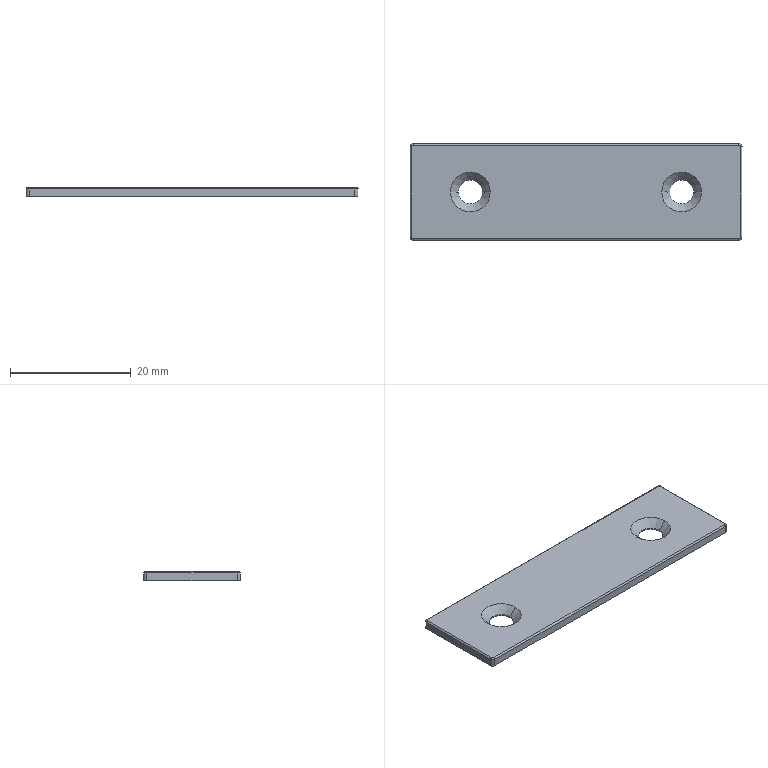Part | SolidWorks | features BaseBody 1 | 1 solid | 26 faces | box 55 x 16 x 1.5 mm | volume 1254 mm3 | cylinder 12 | plane 6 | cone 4 | torus 2 | spline 2 | commonest cylinder face diameters 0.5 x4 1 x4 4 x4
STEP:
#1=CARTESIAN_POINT('',(-15.5,0.,0.2));
#2=VERTEX_POINT('',#1);
#3=CARTESIAN_POINT('',(-19.5,0.,0.2));
#4=VERTEX_POINT('',#3);
#5=CARTESIAN_POINT('',(-17.5,0.,0.2));
#6=DIRECTION('',(0.,0.,-1.));
#7=DIRECTION('',(-1.,0.,0.));
#8=AXIS2_PLACEMENT_3D('',#5,#6,#7);
#9=CIRCLE('',#8,2.);
#10=EDGE_CURVE('',#2,#4,#9,.T.);
#11=ORIENTED_EDGE('',*,*,#10,.F.);
#12=CARTESIAN_POINT('',(-15.5,0.,0.));
#13=VERTEX_POINT('',#12);
#14=CARTESIAN_POINT('',(-15.5,0.,1.5));
#15=DIRECTION('',(0.,0.,-1.));
#16=VECTOR('',#15,1000.);
#17=LINE('',#14,#16);
#18=EDGE_CURVE('',#2,#13,#17,.T.);
#19=ORIENTED_EDGE('',*,*,#18,.T.);
#20=CARTESIAN_POINT('',(-19.5,0.,0.));
#21=VERTEX_POINT('',#20);
#22=CARTESIAN_POINT('',(-17.5,0.,0.));
#23=DIRECTION('',(0.,0.,-1.));
#24=DIRECTION('',(-1.,0.,0.));
#25=AXIS2_PLACEMENT_3D('',#22,#23,#24);
#26=CIRCLE('',#25,2.);
#27=EDGE_CURVE('',#13,#21,#26,.T.);
#28=ORIENTED_EDGE('',*,*,#27,.T.);
#29=CARTESIAN_POINT('',(-19.5,0.,1.5));
#30=DIRECTION('',(0.,0.,-1.));
#31=VECTOR('',#30,1000.);
#32=LINE('',#29,#31);
#33=EDGE_CURVE('',#4,#21,#32,.T.);
#34=ORIENTED_EDGE('',*,*,#33,.F.);
#35=EDGE_LOOP('',(#11,#19,#28,#34));
#36=FACE_OUTER_BOUND('',#35,.T.);
#37=CARTESIAN_POINT('',(-17.5,0.,1.5));
#38=DIRECTION('',(0.,0.,-1.));
#39=DIRECTION('',(-1.,0.,0.));
#40=AXIS2_PLACEMENT_3D('',#37,#38,#39);
#41=CYLINDRICAL_SURFACE('',#40,2.);
#42=ADVANCED_FACE('',(#36),#41,.F.);
#43=CARTESIAN_POINT('',(19.5,0.,0.2));
#44=VERTEX_POINT('',#43);
#45=CARTESIAN_POINT('',(15.5,0.,0.2));
#46=VERTEX_POINT('',#45);
#47=CARTESIAN_POINT('',(17.5,0.,0.2));
#48=DIRECTION('',(0.,0.,-1.));
#49=DIRECTION('',(-1.,0.,0.));
#50=AXIS2_PLACEMENT_3D('',#47,#48,#49);
#51=CIRCLE('',#50,2.);
#52=EDGE_CURVE('',#44,#46,#51,.T.);
#53=ORIENTED_EDGE('',*,*,#52,.F.);
#54=CARTESIAN_POINT('',(19.5,0.,0.));
#55=VERTEX_POINT('',#54);
#56=CARTESIAN_POINT('',(19.5,0.,1.5));
#57=DIRECTION('',(0.,0.,-1.));
#58=VECTOR('',#57,1000.);
#59=LINE('',#56,#58);
#60=EDGE_CURVE('',#44,#55,#59,.T.);
#61=ORIENTED_EDGE('',*,*,#60,.T.);
#62=CARTESIAN_POINT('',(15.5,0.,0.));
#63=VERTEX_POINT('',#62);
#64=CARTESIAN_POINT('',(17.5,0.,0.));
#65=DIRECTION('',(0.,0.,-1.));
#66=DIRECTION('',(-1.,0.,0.));
#67=AXIS2_PLACEMENT_3D('',#64,#65,#66);
#68=CIRCLE('',#67,2.);
#69=EDGE_CURVE('',#55,#63,#68,.T.);
#70=ORIENTED_EDGE('',*,*,#69,.T.);
#71=CARTESIAN_POINT('',(15.5,0.,1.5));
#72=DIRECTION('',(0.,0.,-1.));
#73=VECTOR('',#72,1000.);
#74=LINE('',#71,#73);
#75=EDGE_CURVE('',#46,#63,#74,.T.);
#76=ORIENTED_EDGE('',*,*,#75,.F.);
#77=EDGE_LOOP('',(#53,#61,#70,#76));
#78=FACE_OUTER_BOUND('',#77,.T.);
#79=CARTESIAN_POINT('',(17.5,0.,1.5));
#80=DIRECTION('',(0.,0.,-1.));
#81=DIRECTION('',(-1.,0.,0.));
#82=AXIS2_PLACEMENT_3D('',#79,#80,#81);
#83=CYLINDRICAL_SURFACE('',#82,2.);
#84=ADVANCED_FACE('',(#78),#83,.F.);
#85=ORIENTED_EDGE('',*,*,#10,.T.);
#86=CARTESIAN_POINT('',(-20.8,0.,1.5));
#87=VERTEX_POINT('',#86);
#88=CARTESIAN_POINT('',(-20.8,0.,1.5));
#89=DIRECTION('',(-0.7071,0.,0.7071));
#90=VECTOR('',#89,1000.);
#91=LINE('',#88,#90);
#92=EDGE_CURVE('',#4,#87,#91,.T.);
#93=ORIENTED_EDGE('',*,*,#92,.T.);
#94=CARTESIAN_POINT('',(-14.2,0.,1.5));
#95=VERTEX_POINT('',#94);
#96=CARTESIAN_POINT('',(-17.5,0.,1.5));
#97=DIRECTION('',(0.,0.,-1.));
#98=DIRECTION('',(1.,0.,0.));
#99=AXIS2_PLACEMENT_3D('',#96,#97,#98);
#100=CIRCLE('',#99,3.3);
#101=EDGE_CURVE('',#95,#87,#100,.T.);
#102=ORIENTED_EDGE('',*,*,#101,.F.);
#103=CARTESIAN_POINT('',(-14.2,0.,1.5));
#104=DIRECTION('',(0.7071,0.,0.7071));
#105=VECTOR('',#104,1000.);
#106=LINE('',#103,#105);
#107=EDGE_CURVE('',#2,#95,#106,.T.);
#108=ORIENTED_EDGE('',*,*,#107,.F.);
#109=EDGE_LOOP('',(#85,#93,#102,#108));
#110=FACE_OUTER_BOUND('',#109,.T.);
#111=CARTESIAN_POINT('',(-17.5,0.,1.5));
#112=DIRECTION('',(0.,0.,1.));
#113=DIRECTION('',(1.,0.,0.));
#114=AXIS2_PLACEMENT_3D('',#111,#112,#113);
#115=CONICAL_SURFACE('',#114,3.3,0.7854);
#116=ADVANCED_FACE('',(#110),#115,.F.);
#117=ORIENTED_EDGE('',*,*,#52,.T.);
#118=CARTESIAN_POINT('',(14.2,0.,1.5));
#119=VERTEX_POINT('',#118);
#120=CARTESIAN_POINT('',(14.2,0.,1.5));
#121=DIRECTION('',(-0.7071,0.,0.7071));
#122=VECTOR('',#121,1000.);
#123=LINE('',#120,#122);
#124=EDGE_CURVE('',#46,#119,#123,.T.);
#125=ORIENTED_EDGE('',*,*,#124,.T.);
#126=CARTESIAN_POINT('',(20.8,0.,1.5));
#127=VERTEX_POINT('',#126);
#128=CARTESIAN_POINT('',(17.5,0.,1.5));
#129=DIRECTION('',(0.,0.,-1.));
#130=DIRECTION('',(1.,0.,0.));
#131=AXIS2_PLACEMENT_3D('',#128,#129,#130);
#132=CIRCLE('',#131,3.3);
#133=EDGE_CURVE('',#127,#119,#132,.T.);
#134=ORIENTED_EDGE('',*,*,#133,.F.);
#135=CARTESIAN_POINT('',(20.8,0.,1.5));
#136=DIRECTION('',(0.7071,0.,0.7071));
#137=VECTOR('',#136,1000.);
#138=LINE('',#135,#137);
#139=EDGE_CURVE('',#44,#127,#138,.T.);
#140=ORIENTED_EDGE('',*,*,#139,.F.);
#141=EDGE_LOOP('',(#117,#125,#134,#140));
#142=FACE_OUTER_BOUND('',#141,.T.);
#143=CARTESIAN_POINT('',(17.5,0.,1.5));
#144=DIRECTION('',(0.,0.,1.));
#145=DIRECTION('',(1.,0.,0.));
#146=AXIS2_PLACEMENT_3D('',#143,#144,#145);
#147=CONICAL_SURFACE('',#146,3.3,0.7854);
#148=ADVANCED_FACE('',(#142),#147,.F.);
#149=CARTESIAN_POINT('',(-17.5,0.,0.));
#150=DIRECTION('',(0.,0.,-1.));
#151=DIRECTION('',(-1.,0.,0.));
#152=AXIS2_PLACEMENT_3D('',#149,#150,#151);
#153=CIRCLE('',#152,2.);
#154=EDGE_CURVE('',#21,#13,#153,.T.);
#155=ORIENTED_EDGE('',*,*,#154,.F.);
#156=ORIENTED_EDGE('',*,*,#27,.F.);
#157=EDGE_LOOP('',(#155,#156));
#158=FACE_BOUND('',#157,.T.);
#159=CARTESIAN_POINT('',(17.5,0.,0.));
#160=DIRECTION('',(0.,0.,-1.));
#161=DIRECTION('',(-1.,0.,0.));
#162=AXIS2_PLACEMENT_3D('',#159,#160,#161);
#163=CIRCLE('',#162,2.);
#164=EDGE_CURVE('',#63,#55,#163,.T.);
#165=ORIENTED_EDGE('',*,*,#164,.F.);
#166=ORIENTED_EDGE('',*,*,#69,.F.);
#167=EDGE_LOOP('',(#165,#166));
#168=FACE_BOUND('',#167,.T.);
#169=CARTESIAN_POINT('',(-27.5,-7.5,0.));
#170=VERTEX_POINT('',#169);
#171=CARTESIAN_POINT('',(-27.,-8.,0.));
#172=VERTEX_POINT('',#171);
#173=CARTESIAN_POINT('',(-27.,-7.5,0.));
#174=DIRECTION('',(0.,0.,1.));
#175=DIRECTION('',(-1.,0.,0.));
#176=AXIS2_PLACEMENT_3D('',#173,#174,#175);
#177=CIRCLE('',#176,0.5);
#178=EDGE_CURVE('',#170,#172,#177,.T.);
#179=ORIENTED_EDGE('',*,*,#178,.F.);
#180=CARTESIAN_POINT('',(-27.5,7.5,0.));
#181=VERTEX_POINT('',#180);
#182=CARTESIAN_POINT('',(-27.5,0.,0.));
#183=DIRECTION('',(0.,-1.,0.));
#184=VECTOR('',#183,1000.);
#185=LINE('',#182,#184);
#186=EDGE_CURVE('',#181,#170,#185,.T.);
#187=ORIENTED_EDGE('',*,*,#186,.F.);
#188=CARTESIAN_POINT('',(-27.,8.,0.));
#189=VERTEX_POINT('',#188);
#190=CARTESIAN_POINT('',(-27.,7.5,0.));
#191=DIRECTION('',(0.,0.,1.));
#192=DIRECTION('',(-1.,0.,0.));
#193=AXIS2_PLACEMENT_3D('',#190,#191,#192);
#194=CIRCLE('',#193,0.5);
#195=EDGE_CURVE('',#189,#181,#194,.T.);
#196=ORIENTED_EDGE('',*,*,#195,.F.);
#197=CARTESIAN_POINT('',(27.,8.,0.));
#198=VERTEX_POINT('',#197);
#199=CARTESIAN_POINT('',(0.,8.,0.));
#200=DIRECTION('',(-1.,0.,0.));
#201=VECTOR('',#200,1000.);
#202=LINE('',#199,#201);
#203=EDGE_CURVE('',#198,#189,#202,.T.);
#204=ORIENTED_EDGE('',*,*,#203,.F.);
#205=CARTESIAN_POINT('',(27.5,7.5,0.));
#206=VERTEX_POINT('',#205);
#207=CARTESIAN_POINT('',(27.,7.5,0.));
#208=DIRECTION('',(0.,0.,1.));
#209=DIRECTION('',(-1.,0.,0.));
#210=AXIS2_PLACEMENT_3D('',#207,#208,#209);
#211=CIRCLE('',#210,0.5);
#212=EDGE_CURVE('',#206,#198,#211,.T.);
#213=ORIENTED_EDGE('',*,*,#212,.F.);
#214=CARTESIAN_POINT('',(27.5,-7.5,0.));
#215=VERTEX_POINT('',#214);
#216=CARTESIAN_POINT('',(27.5,0.,0.));
#217=DIRECTION('',(0.,1.,0.));
#218=VECTOR('',#217,1000.);
#219=LINE('',#216,#218);
#220=EDGE_CURVE('',#215,#206,#219,.T.);
#221=ORIENTED_EDGE('',*,*,#220,.F.);
#222=CARTESIAN_POINT('',(27.,-8.,0.));
#223=VERTEX_POINT('',#222);
#224=CARTESIAN_POINT('',(27.,-7.5,0.));
#225=DIRECTION('',(0.,0.,1.));
#226=DIRECTION('',(-1.,0.,0.));
#227=AXIS2_PLACEMENT_3D('',#224,#225,#226);
#228=CIRCLE('',#227,0.5);
#229=EDGE_CURVE('',#223,#215,#228,.T.);
#230=ORIENTED_EDGE('',*,*,#229,.F.);
#231=CARTESIAN_POINT('',(0.,-8.,0.));
#232=DIRECTION('',(1.,0.,0.));
#233=VECTOR('',#232,1000.);
#234=LINE('',#231,#233);
#235=EDGE_CURVE('',#172,#223,#234,.T.);
#236=ORIENTED_EDGE('',*,*,#235,.F.);
#237=EDGE_LOOP('',(#179,#187,#196,#204,#213,#221,#230,#236));
#238=FACE_OUTER_BOUND('',#237,.T.);
#239=CARTESIAN_POINT('',(0.,0.,0.));
#240=DIRECTION('',(0.,0.,1.));
#241=DIRECTION('',(1.,0.,0.));
#242=AXIS2_PLACEMENT_3D('',#239,#240,#241);
#243=PLANE('',#242);
#244=ADVANCED_FACE('',(#158,#168,#238),#243,.F.);
#245=ORIENTED_EDGE('',*,*,#18,.F.);
#246=CARTESIAN_POINT('',(-17.5,0.,0.2));
#247=DIRECTION('',(0.,0.,-1.));
#248=DIRECTION('',(-1.,0.,0.));
#249=AXIS2_PLACEMENT_3D('',#246,#247,#248);
#250=CIRCLE('',#249,2.);
#251=EDGE_CURVE('',#4,#2,#250,.T.);
#252=ORIENTED_EDGE('',*,*,#251,.F.);
#253=ORIENTED_EDGE('',*,*,#33,.T.);
#254=ORIENTED_EDGE('',*,*,#154,.T.);
#255=EDGE_LOOP('',(#245,#252,#253,#254));
#256=FACE_OUTER_BOUND('',#255,.T.);
#257=CARTESIAN_POINT('',(-17.5,0.,1.5));
#258=DIRECTION('',(0.,0.,-1.));
#259=DIRECTION('',(-1.,0.,0.));
#260=AXIS2_PLACEMENT_3D('',#257,#258,#259);
#261=CYLINDRICAL_SURFACE('',#260,2.);
#262=ADVANCED_FACE('',(#256),#261,.F.);
#263=ORIENTED_EDGE('',*,*,#60,.F.);
#264=CARTESIAN_POINT('',(17.5,0.,0.2));
#265=DIRECTION('',(0.,0.,-1.));
#266=DIRECTION('',(-1.,0.,0.));
#267=AXIS2_PLACEMENT_3D('',#264,#265,#266);
#268=CIRCLE('',#267,2.);
#269=EDGE_CURVE('',#46,#44,#268,.T.);
#270=ORIENTED_EDGE('',*,*,#269,.F.);
#271=ORIENTED_EDGE('',*,*,#75,.T.);
#272=ORIENTED_EDGE('',*,*,#164,.T.);
#273=EDGE_LOOP('',(#263,#270,#271,#272));
#274=FACE_OUTER_BOUND('',#273,.T.);
#275=CARTESIAN_POINT('',(17.5,0.,1.5));
#276=DIRECTION('',(0.,0.,-1.));
#277=DIRECTION('',(-1.,0.,0.));
#278=AXIS2_PLACEMENT_3D('',#275,#276,#277);
#279=CYLINDRICAL_SURFACE('',#278,2.);
#280=ADVANCED_FACE('',(#274),#279,.F.);
#281=CARTESIAN_POINT('',(27.,-8.,1.25));
#282=VERTEX_POINT('',#281);
#283=CARTESIAN_POINT('',(27.,-8.,0.));
#284=DIRECTION('',(0.,0.,1.));
#285=VECTOR('',#284,1000.);
#286=LINE('',#283,#285);
#287=EDGE_CURVE('',#223,#282,#286,.T.);
#288=ORIENTED_EDGE('',*,*,#287,.T.);
#289=CARTESIAN_POINT('',(-27.,-8.,1.25));
#290=VERTEX_POINT('',#289);
#291=CARTESIAN_POINT('',(-27.5,-8.,1.25));
#292=DIRECTION('',(-1.,0.,0.));
#293=VECTOR('',#292,1000.);
#294=LINE('',#291,#293);
#295=EDGE_CURVE('',#282,#290,#294,.T.);
#296=ORIENTED_EDGE('',*,*,#295,.T.);
#297=CARTESIAN_POINT('',(-27.,-8.,0.));
#298=DIRECTION('',(0.,0.,-1.));
#299=VECTOR('',#298,1000.);
#300=LINE('',#297,#299);
#301=EDGE_CURVE('',#290,#172,#300,.T.);
#302=ORIENTED_EDGE('',*,*,#301,.T.);
#303=ORIENTED_EDGE('',*,*,#235,.T.);
#304=EDGE_LOOP('',(#288,#296,#302,#303));
#305=FACE_OUTER_BOUND('',#304,.T.);
#306=CARTESIAN_POINT('',(-27.5,-8.,0.));
#307=DIRECTION('',(0.,-1.,0.));
#308=DIRECTION('',(0.,0.,-1.));
#309=AXIS2_PLACEMENT_3D('',#306,#307,#308);
#310=PLANE('',#309);
#311=ADVANCED_FACE('',(#305),#310,.T.);
#312=ORIENTED_EDGE('',*,*,#301,.F.);
#313=CARTESIAN_POINT('',(-27.5,-7.5,1.25));
#314=VERTEX_POINT('',#313);
#315=CARTESIAN_POINT('',(-27.,-7.5,1.25));
#316=DIRECTION('',(0.,0.,-1.));
#317=DIRECTION('',(-1.,0.,0.));
#318=AXIS2_PLACEMENT_3D('',#315,#316,#317);
#319=CIRCLE('',#318,0.5);
#320=EDGE_CURVE('',#290,#314,#319,.T.);
#321=ORIENTED_EDGE('',*,*,#320,.T.);
#322=CARTESIAN_POINT('',(-27.5,-7.5,0.));
#323=DIRECTION('',(0.,0.,-1.));
#324=VECTOR('',#323,1000.);
#325=LINE('',#322,#324);
#326=EDGE_CURVE('',#314,#170,#325,.T.);
#327=ORIENTED_EDGE('',*,*,#326,.T.);
#328=ORIENTED_EDGE('',*,*,#178,.T.);
#329=EDGE_LOOP('',(#312,#321,#327,#328));
#330=FACE_OUTER_BOUND('',#329,.T.);
#331=CARTESIAN_POINT('',(-27.,-7.5,1.599));
#332=DIRECTION('',(0.,0.,-1.));
#333=DIRECTION('',(-1.,0.,0.));
#334=AXIS2_PLACEMENT_3D('',#331,#332,#333);
#335=CYLINDRICAL_SURFACE('',#334,0.5);
#336=ADVANCED_FACE('',(#330),#335,.T.);
#337=ORIENTED_EDGE('',*,*,#326,.F.);
#338=CARTESIAN_POINT('',(-27.5,7.5,1.25));
#339=VERTEX_POINT('',#338);
#340=CARTESIAN_POINT('',(-27.5,8.,1.25));
#341=DIRECTION('',(0.,1.,0.));
#342=VECTOR('',#341,1000.);
#343=LINE('',#340,#342);
#344=EDGE_CURVE('',#314,#339,#343,.T.);
#345=ORIENTED_EDGE('',*,*,#344,.T.);
#346=CARTESIAN_POINT('',(-27.5,7.5,0.));
#347=DIRECTION('',(0.,0.,-1.));
#348=VECTOR('',#347,1000.);
#349=LINE('',#346,#348);
#350=EDGE_CURVE('',#339,#181,#349,.T.);
#351=ORIENTED_EDGE('',*,*,#350,.T.);
#352=ORIENTED_EDGE('',*,*,#186,.T.);
#353=EDGE_LOOP('',(#337,#345,#351,#352));
#354=FACE_OUTER_BOUND('',#353,.T.);
#355=CARTESIAN_POINT('',(-27.5,8.,0.));
#356=DIRECTION('',(-1.,0.,0.));
#357=DIRECTION('',(0.,0.,1.));
#358=AXIS2_PLACEMENT_3D('',#355,#356,#357);
#359=PLANE('',#358);
#360=ADVANCED_FACE('',(#354),#359,.T.);
#361=ORIENTED_EDGE('',*,*,#350,.F.);
#362=CARTESIAN_POINT('',(-27.,8.,1.25));
#363=VERTEX_POINT('',#362);
#364=CARTESIAN_POINT('',(-27.,7.5,1.25));
#365=DIRECTION('',(0.,0.,-1.));
#366=DIRECTION('',(-1.,0.,0.));
#367=AXIS2_PLACEMENT_3D('',#364,#365,#366);
#368=CIRCLE('',#367,0.5);
#369=EDGE_CURVE('',#339,#363,#368,.T.);
#370=ORIENTED_EDGE('',*,*,#369,.T.);
#371=CARTESIAN_POINT('',(-27.,8.,1.599));
#372=DIRECTION('',(0.,0.,-1.));
#373=VECTOR('',#372,1000.);
#374=LINE('',#371,#373);
#375=EDGE_CURVE('',#363,#189,#374,.T.);
#376=ORIENTED_EDGE('',*,*,#375,.T.);
#377=ORIENTED_EDGE('',*,*,#195,.T.);
#378=EDGE_LOOP('',(#361,#370,#376,#377));
#379=FACE_OUTER_BOUND('',#378,.T.);
#380=CARTESIAN_POINT('',(-27.,7.5,1.599));
#381=DIRECTION('',(0.,0.,-1.));
#382=DIRECTION('',(-1.,0.,0.));
#383=AXIS2_PLACEMENT_3D('',#380,#381,#382);
#384=CYLINDRICAL_SURFACE('',#383,0.5);
#385=ADVANCED_FACE('',(#379),#384,.T.);
#386=ORIENTED_EDGE('',*,*,#375,.F.);
#387=CARTESIAN_POINT('',(27.,8.,1.25));
#388=VERTEX_POINT('',#387);
#389=CARTESIAN_POINT('',(27.5,8.,1.25));
#390=DIRECTION('',(1.,0.,0.));
#391=VECTOR('',#390,1000.);
#392=LINE('',#389,#391);
#393=EDGE_CURVE('',#363,#388,#392,.T.);
#394=ORIENTED_EDGE('',*,*,#393,.T.);
#395=CARTESIAN_POINT('',(27.,8.,0.));
#396=DIRECTION('',(0.,0.,-1.));
#397=VECTOR('',#396,1000.);
#398=LINE('',#395,#397);
#399=EDGE_CURVE('',#388,#198,#398,.T.);
#400=ORIENTED_EDGE('',*,*,#399,.T.);
#401=ORIENTED_EDGE('',*,*,#203,.T.);
#402=EDGE_LOOP('',(#386,#394,#400,#401));
#403=FACE_OUTER_BOUND('',#402,.T.);
#404=CARTESIAN_POINT('',(27.5,8.,0.));
#405=DIRECTION('',(0.,1.,0.));
#406=DIRECTION('',(0.,0.,1.));
#407=AXIS2_PLACEMENT_3D('',#404,#405,#406);
#408=PLANE('',#407);
#409=ADVANCED_FACE('',(#403),#408,.T.);
#410=ORIENTED_EDGE('',*,*,#399,.F.);
#411=CARTESIAN_POINT('',(27.5,7.5,1.25));
#412=VERTEX_POINT('',#411);
#413=CARTESIAN_POINT('',(27.,7.5,1.25));
#414=DIRECTION('',(0.,0.,-1.));
#415=DIRECTION('',(-1.,0.,0.));
#416=AXIS2_PLACEMENT_3D('',#413,#414,#415);
#417=CIRCLE('',#416,0.5);
#418=EDGE_CURVE('',#388,#412,#417,.T.);
#419=ORIENTED_EDGE('',*,*,#418,.T.);
#420=CARTESIAN_POINT('',(27.5,7.5,1.599));
#421=DIRECTION('',(0.,0.,-1.));
#422=VECTOR('',#421,1000.);
#423=LINE('',#420,#422);
#424=EDGE_CURVE('',#412,#206,#423,.T.);
#425=ORIENTED_EDGE('',*,*,#424,.T.);
#426=ORIENTED_EDGE('',*,*,#212,.T.);
#427=EDGE_LOOP('',(#410,#419,#425,#426));
#428=FACE_OUTER_BOUND('',#427,.T.);
#429=CARTESIAN_POINT('',(27.,7.5,1.599));
#430=DIRECTION('',(0.,0.,-1.));
#431=DIRECTION('',(-1.,0.,0.));
#432=AXIS2_PLACEMENT_3D('',#429,#430,#431);
#433=CYLINDRICAL_SURFACE('',#432,0.5);
#434=ADVANCED_FACE('',(#428),#433,.T.);
#435=ORIENTED_EDGE('',*,*,#424,.F.);
#436=CARTESIAN_POINT('',(27.5,-7.5,1.25));
#437=VERTEX_POINT('',#436);
#438=CARTESIAN_POINT('',(27.5,-8.,1.25));
#439=DIRECTION('',(0.,-1.,0.));
#440=VECTOR('',#439,1000.);
#441=LINE('',#438,#440);
#442=EDGE_CURVE('',#412,#437,#441,.T.);
#443=ORIENTED_EDGE('',*,*,#442,.T.);
#444=CARTESIAN_POINT('',(27.5,-7.5,0.));
#445=DIRECTION('',(0.,0.,-1.));
#446=VECTOR('',#445,1000.);
#447=LINE('',#444,#446);
#448=EDGE_CURVE('',#437,#215,#447,.T.);
#449=ORIENTED_EDGE('',*,*,#448,.T.);
#450=ORIENTED_EDGE('',*,*,#220,.T.);
#451=EDGE_LOOP('',(#435,#443,#449,#450));
#452=FACE_OUTER_BOUND('',#451,.T.);
#453=CARTESIAN_POINT('',(27.5,-8.,0.));
#454=DIRECTION('',(1.,0.,0.));
#455=DIRECTION('',(0.,0.,-1.));
#456=AXIS2_PLACEMENT_3D('',#453,#454,#455);
#457=PLANE('',#456);
#458=ADVANCED_FACE('',(#452),#457,.T.);
#459=ORIENTED_EDGE('',*,*,#448,.F.);
#460=CARTESIAN_POINT('',(27.,-7.5,1.25));
#461=DIRECTION('',(0.,0.,-1.));
#462=DIRECTION('',(-1.,0.,0.));
#463=AXIS2_PLACEMENT_3D('',#460,#461,#462);
#464=CIRCLE('',#463,0.5);
#465=EDGE_CURVE('',#437,#282,#464,.T.);
#466=ORIENTED_EDGE('',*,*,#465,.T.);
#467=ORIENTED_EDGE('',*,*,#287,.F.);
#468=ORIENTED_EDGE('',*,*,#229,.T.);
#469=EDGE_LOOP('',(#459,#466,#467,#468));
#470=FACE_OUTER_BOUND('',#469,.T.);
#471=CARTESIAN_POINT('',(27.,-7.5,1.599));
#472=DIRECTION('',(0.,0.,-1.));
#473=DIRECTION('',(-1.,0.,0.));
#474=AXIS2_PLACEMENT_3D('',#471,#472,#473);
#475=CYLINDRICAL_SURFACE('',#474,0.5);
#476=ADVANCED_FACE('',(#470),#475,.T.);
#477=ORIENTED_EDGE('',*,*,#92,.F.);
#478=ORIENTED_EDGE('',*,*,#251,.T.);
#479=ORIENTED_EDGE('',*,*,#107,.T.);
#480=CARTESIAN_POINT('',(-17.5,0.,1.5));
#481=DIRECTION('',(0.,0.,-1.));
#482=DIRECTION('',(1.,0.,0.));
#483=AXIS2_PLACEMENT_3D('',#480,#481,#482);
#484=CIRCLE('',#483,3.3);
#485=EDGE_CURVE('',#87,#95,#484,.T.);
#486=ORIENTED_EDGE('',*,*,#485,.F.);
#487=EDGE_LOOP('',(#477,#478,#479,#486));
#488=FACE_OUTER_BOUND('',#487,.T.);
#489=CARTESIAN_POINT('',(-17.5,0.,1.5));
#490=DIRECTION('',(0.,0.,1.));
#491=DIRECTION('',(1.,0.,0.));
#492=AXIS2_PLACEMENT_3D('',#489,#490,#491);
#493=CONICAL_SURFACE('',#492,3.3,0.7854);
#494=ADVANCED_FACE('',(#488),#493,.F.);
#495=ORIENTED_EDGE('',*,*,#124,.F.);
#496=ORIENTED_EDGE('',*,*,#269,.T.);
#497=ORIENTED_EDGE('',*,*,#139,.T.);
#498=CARTESIAN_POINT('',(17.5,0.,1.5));
#499=DIRECTION('',(0.,0.,-1.));
#500=DIRECTION('',(1.,0.,0.));
#501=AXIS2_PLACEMENT_3D('',#498,#499,#500);
#502=CIRCLE('',#501,3.3);
#503=EDGE_CURVE('',#119,#127,#502,.T.);
#504=ORIENTED_EDGE('',*,*,#503,.F.);
#505=EDGE_LOOP('',(#495,#496,#497,#504));
#506=FACE_OUTER_BOUND('',#505,.T.);
#507=CARTESIAN_POINT('',(17.5,0.,1.5));
#508=DIRECTION('',(0.,0.,1.));
#509=DIRECTION('',(1.,0.,0.));
#510=AXIS2_PLACEMENT_3D('',#507,#508,#509);
#511=CONICAL_SURFACE('',#510,3.3,0.7854);
#512=ADVANCED_FACE('',(#506),#511,.F.);
#513=CARTESIAN_POINT('',(27.,-7.75,1.5));
#514=VERTEX_POINT('',#513);
#515=CARTESIAN_POINT('',(27.,-7.75,1.25));
#516=DIRECTION('',(-1.,0.,0.));
#517=DIRECTION('',(0.,0.,-1.));
#518=AXIS2_PLACEMENT_3D('',#515,#516,#517);
#519=CIRCLE('',#518,0.25);
#520=EDGE_CURVE('',#282,#514,#519,.T.);
#521=ORIENTED_EDGE('',*,*,#520,.T.);
#522=CARTESIAN_POINT('',(-27.,-7.75,1.5));
#523=VERTEX_POINT('',#522);
#524=CARTESIAN_POINT('',(-27.097,-7.75,1.5));
#525=DIRECTION('',(-1.,0.,0.));
#526=VECTOR('',#525,1000.);
#527=LINE('',#524,#526);
#528=EDGE_CURVE('',#514,#523,#527,.T.);
#529=ORIENTED_EDGE('',*,*,#528,.T.);
#530=CARTESIAN_POINT('',(-27.,-7.75,1.25));
#531=DIRECTION('',(1.,0.,0.));
#532=DIRECTION('',(0.,0.,-1.));
#533=AXIS2_PLACEMENT_3D('',#530,#531,#532);
#534=CIRCLE('',#533,0.25);
#535=EDGE_CURVE('',#523,#290,#534,.T.);
#536=ORIENTED_EDGE('',*,*,#535,.T.);
#537=ORIENTED_EDGE('',*,*,#295,.F.);
#538=EDGE_LOOP('',(#521,#529,#536,#537));
#539=FACE_OUTER_BOUND('',#538,.T.);
#540=CARTESIAN_POINT('',(-27.097,-7.75,1.25));
#541=DIRECTION('',(1.,0.,0.));
#542=DIRECTION('',(0.,0.,-1.));
#543=AXIS2_PLACEMENT_3D('',#540,#541,#542);
#544=CYLINDRICAL_SURFACE('',#543,0.25);
#545=ADVANCED_FACE('',(#539),#544,.T.);
#546=ORIENTED_EDGE('',*,*,#535,.F.);
#547=CARTESIAN_POINT('',(-27.25,-7.5,1.5));
#548=VERTEX_POINT('',#547);
#549=CARTESIAN_POINT('',(-27.,-7.75,1.5));
#550=CARTESIAN_POINT('',(-27.04,-7.75,1.5));
#551=CARTESIAN_POINT('',(-27.075,-7.74,1.5));
#552=CARTESIAN_POINT('',(-27.117,-7.722,1.5));
#553=CARTESIAN_POINT('',(-27.129,-7.715,1.5));
#554=CARTESIAN_POINT('',(-27.151,-7.7,1.5));
#555=CARTESIAN_POINT('',(-27.164,-7.69,1.5));
#556=CARTESIAN_POINT('',(-27.199,-7.655,1.5));
#557=CARTESIAN_POINT('',(-27.219,-7.625,1.5));
#558=CARTESIAN_POINT('',(-27.244,-7.565,1.5));
#559=CARTESIAN_POINT('',(-27.251,-7.532,1.5));
#560=CARTESIAN_POINT('',(-27.25,-7.5,1.5));
#561=B_SPLINE_CURVE_WITH_KNOTS('',3,(#549,#550,#551,#552,#553,#554,#555,#556,#557,#558,#559,#560),.UNSPECIFIED.,.F.,.F.,(4,2,2,2,2,4),(0.,0.25,0.375,0.5,0.75,1.),.UNSPECIFIED.);
#562=EDGE_CURVE('',#523,#548,#561,.T.);
#563=ORIENTED_EDGE('',*,*,#562,.T.);
#564=CARTESIAN_POINT('',(-27.25,-7.5,1.25));
#565=DIRECTION('',(0.,-1.,0.));
#566=DIRECTION('',(0.,0.,-1.));
#567=AXIS2_PLACEMENT_3D('',#564,#565,#566);
#568=CIRCLE('',#567,0.25);
#569=EDGE_CURVE('',#548,#314,#568,.T.);
#570=ORIENTED_EDGE('',*,*,#569,.T.);
#571=ORIENTED_EDGE('',*,*,#320,.F.);
#572=EDGE_LOOP('',(#546,#563,#570,#571));
#573=FACE_OUTER_BOUND('',#572,.T.);
#574=CARTESIAN_POINT('',(-27.,-7.5,1.25));
#575=DIRECTION('',(0.,0.,-1.));
#576=DIRECTION('',(-1.,0.,0.));
#577=AXIS2_PLACEMENT_3D('',#574,#575,#576);
#578=TOROIDAL_SURFACE('',#577,0.25,0.25);
#579=ADVANCED_FACE('',(#573),#578,.T.);
#580=ORIENTED_EDGE('',*,*,#569,.F.);
#581=CARTESIAN_POINT('',(-27.25,7.5,1.5));
#582=VERTEX_POINT('',#581);
#583=CARTESIAN_POINT('',(-27.25,7.597,1.5));
#584=DIRECTION('',(0.,1.,0.));
#585=VECTOR('',#584,1000.);
#586=LINE('',#583,#585);
#587=EDGE_CURVE('',#548,#582,#586,.T.);
#588=ORIENTED_EDGE('',*,*,#587,.T.);
#589=CARTESIAN_POINT('',(-27.25,7.5,1.25));
#590=DIRECTION('',(0.,-1.,0.));
#591=DIRECTION('',(0.,0.,-1.));
#592=AXIS2_PLACEMENT_3D('',#589,#590,#591);
#593=CIRCLE('',#592,0.25);
#594=EDGE_CURVE('',#582,#339,#593,.T.);
#595=ORIENTED_EDGE('',*,*,#594,.T.);
#596=ORIENTED_EDGE('',*,*,#344,.F.);
#597=EDGE_LOOP('',(#580,#588,#595,#596));
#598=FACE_OUTER_BOUND('',#597,.T.);
#599=CARTESIAN_POINT('',(-27.25,7.597,1.25));
#600=DIRECTION('',(0.,-1.,0.));
#601=DIRECTION('',(0.,0.,-1.));
#602=AXIS2_PLACEMENT_3D('',#599,#600,#601);
#603=CYLINDRICAL_SURFACE('',#602,0.25);
#604=ADVANCED_FACE('',(#598),#603,.T.);
#605=ORIENTED_EDGE('',*,*,#594,.F.);
#606=CARTESIAN_POINT('',(-27.,7.75,1.5));
#607=VERTEX_POINT('',#606);
#608=CARTESIAN_POINT('',(-27.25,7.5,1.5));
#609=CARTESIAN_POINT('',(-27.25,7.646,1.5));
#610=CARTESIAN_POINT('',(-27.146,7.75,1.5));
#611=CARTESIAN_POINT('',(-27.,7.75,1.5));
#612=(BOUNDED_CURVE()B_SPLINE_CURVE(3,(#608,#609,#610,#611),.UNSPECIFIED.,.F.,.T.)B_SPLINE_CURVE_WITH_KNOTS((4,4),(0.,1.),.UNSPECIFIED.)CURVE()GEOMETRIC_REPRESENTATION_ITEM()RATIONAL_B_SPLINE_CURVE((1.,0.8047,0.8047,1.))REPRESENTATION_ITEM(''));
#613=EDGE_CURVE('',#582,#607,#612,.T.);
#614=ORIENTED_EDGE('',*,*,#613,.T.);
#615=CARTESIAN_POINT('',(-27.,7.75,1.25));
#616=DIRECTION('',(-1.,0.,0.));
#617=DIRECTION('',(0.,1.,0.));
#618=AXIS2_PLACEMENT_3D('',#615,#616,#617);
#619=CIRCLE('',#618,0.25);
#620=EDGE_CURVE('',#607,#363,#619,.T.);
#621=ORIENTED_EDGE('',*,*,#620,.T.);
#622=ORIENTED_EDGE('',*,*,#369,.F.);
#623=EDGE_LOOP('',(#605,#614,#621,#622));
#624=FACE_OUTER_BOUND('',#623,.T.);
#625=CARTESIAN_POINT('',(-27.5,7.5,1.25));
#626=CARTESIAN_POINT('',(-27.5,7.793,1.25));
#627=CARTESIAN_POINT('',(-27.293,8.,1.25));
#628=CARTESIAN_POINT('',(-27.,8.,1.25));
#629=CARTESIAN_POINT('',(-27.5,7.5,1.396));
#630=CARTESIAN_POINT('',(-27.5,7.793,1.396));
#631=CARTESIAN_POINT('',(-27.293,8.,1.396));
#632=CARTESIAN_POINT('',(-27.,8.,1.396));
#633=CARTESIAN_POINT('',(-27.396,7.5,1.5));
#634=CARTESIAN_POINT('',(-27.396,7.732,1.5));
#635=CARTESIAN_POINT('',(-27.232,7.896,1.5));
#636=CARTESIAN_POINT('',(-27.,7.896,1.5));
#637=CARTESIAN_POINT('',(-27.25,7.5,1.5));
#638=CARTESIAN_POINT('',(-27.25,7.646,1.5));
#639=CARTESIAN_POINT('',(-27.146,7.75,1.5));
#640=CARTESIAN_POINT('',(-27.,7.75,1.5));
#641=(BOUNDED_SURFACE()B_SPLINE_SURFACE(3,3,((#625,#626,#627,#628),(#629,#630,#631,#632),(#633,#634,#635,#636),(#637,#638,#639,#640)),.UNSPECIFIED.,.F.,.F.,.T.)B_SPLINE_SURFACE_WITH_KNOTS((4,4),(4,4),(0.,1.),(0.,1.),.UNSPECIFIED.)GEOMETRIC_REPRESENTATION_ITEM()RATIONAL_B_SPLINE_SURFACE(((1.,0.8047,0.8047,1.),(0.8047,0.6476,0.6476,0.8047),(0.8047,0.6476,0.6476,0.8047),(1.,0.8047,0.8047,1.)))REPRESENTATION_ITEM('')SURFACE());
#642=ADVANCED_FACE('',(#624),#641,.T.);
#643=ORIENTED_EDGE('',*,*,#620,.F.);
#644=CARTESIAN_POINT('',(27.,7.75,1.5));
#645=VERTEX_POINT('',#644);
#646=CARTESIAN_POINT('',(27.097,7.75,1.5));
#647=DIRECTION('',(1.,0.,0.));
#648=VECTOR('',#647,1000.);
#649=LINE('',#646,#648);
#650=EDGE_CURVE('',#607,#645,#649,.T.);
#651=ORIENTED_EDGE('',*,*,#650,.T.);
#652=CARTESIAN_POINT('',(27.,7.75,1.25));
#653=DIRECTION('',(-1.,0.,0.));
#654=DIRECTION('',(0.,0.,1.));
#655=AXIS2_PLACEMENT_3D('',#652,#653,#654);
#656=CIRCLE('',#655,0.25);
#657=EDGE_CURVE('',#645,#388,#656,.T.);
#658=ORIENTED_EDGE('',*,*,#657,.T.);
#659=ORIENTED_EDGE('',*,*,#393,.F.);
#660=EDGE_LOOP('',(#643,#651,#658,#659));
#661=FACE_OUTER_BOUND('',#660,.T.);
#662=CARTESIAN_POINT('',(27.097,7.75,1.25));
#663=DIRECTION('',(-1.,0.,0.));
#664=DIRECTION('',(0.,0.,1.));
#665=AXIS2_PLACEMENT_3D('',#662,#663,#664);
#666=CYLINDRICAL_SURFACE('',#665,0.25);
#667=ADVANCED_FACE('',(#661),#666,.T.);
#668=ORIENTED_EDGE('',*,*,#657,.F.);
#669=CARTESIAN_POINT('',(27.25,7.5,1.5));
#670=VERTEX_POINT('',#669);
#671=CARTESIAN_POINT('',(27.,7.75,1.5));
#672=CARTESIAN_POINT('',(27.04,7.75,1.5));
#673=CARTESIAN_POINT('',(27.075,7.74,1.5));
#674=CARTESIAN_POINT('',(27.117,7.722,1.5));
#675=CARTESIAN_POINT('',(27.129,7.715,1.5));
#676=CARTESIAN_POINT('',(27.151,7.7,1.5));
#677=CARTESIAN_POINT('',(27.164,7.69,1.5));
#678=CARTESIAN_POINT('',(27.199,7.655,1.5));
#679=CARTESIAN_POINT('',(27.219,7.625,1.5));
#680=CARTESIAN_POINT('',(27.244,7.565,1.5));
#681=CARTESIAN_POINT('',(27.251,7.532,1.5));
#682=CARTESIAN_POINT('',(27.25,7.5,1.5));
#683=B_SPLINE_CURVE_WITH_KNOTS('',3,(#671,#672,#673,#674,#675,#676,#677,#678,#679,#680,#681,#682),.UNSPECIFIED.,.F.,.F.,(4,2,2,2,2,4),(0.,0.25,0.375,0.5,0.75,1.),.UNSPECIFIED.);
#684=EDGE_CURVE('',#645,#670,#683,.T.);
#685=ORIENTED_EDGE('',*,*,#684,.T.);
#686=CARTESIAN_POINT('',(27.25,7.5,1.25));
#687=DIRECTION('',(0.,1.,0.));
#688=DIRECTION('',(0.,0.,1.));
#689=AXIS2_PLACEMENT_3D('',#686,#687,#688);
#690=CIRCLE('',#689,0.25);
#691=EDGE_CURVE('',#670,#412,#690,.T.);
#692=ORIENTED_EDGE('',*,*,#691,.T.);
#693=ORIENTED_EDGE('',*,*,#418,.F.);
#694=EDGE_LOOP('',(#668,#685,#692,#693));
#695=FACE_OUTER_BOUND('',#694,.T.);
#696=CARTESIAN_POINT('',(27.,7.5,1.25));
#697=DIRECTION('',(0.,0.,-1.));
#698=DIRECTION('',(-1.,0.,0.));
#699=AXIS2_PLACEMENT_3D('',#696,#697,#698);
#700=TOROIDAL_SURFACE('',#699,0.25,0.25);
#701=ADVANCED_FACE('',(#695),#700,.T.);
#702=ORIENTED_EDGE('',*,*,#691,.F.);
#703=CARTESIAN_POINT('',(27.25,-7.5,1.5));
#704=VERTEX_POINT('',#703);
#705=CARTESIAN_POINT('',(27.25,0.,1.5));
#706=DIRECTION('',(0.,-1.,0.));
#707=VECTOR('',#706,1000.);
#708=LINE('',#705,#707);
#709=EDGE_CURVE('',#670,#704,#708,.T.);
#710=ORIENTED_EDGE('',*,*,#709,.T.);
#711=CARTESIAN_POINT('',(27.25,-7.5,1.25));
#712=DIRECTION('',(0.,1.,0.));
#713=DIRECTION('',(0.,0.,1.));
#714=AXIS2_PLACEMENT_3D('',#711,#712,#713);
#715=CIRCLE('',#714,0.25);
#716=EDGE_CURVE('',#704,#437,#715,.T.);
#717=ORIENTED_EDGE('',*,*,#716,.T.);
#718=ORIENTED_EDGE('',*,*,#442,.F.);
#719=EDGE_LOOP('',(#702,#710,#717,#718));
#720=FACE_OUTER_BOUND('',#719,.T.);
#721=CARTESIAN_POINT('',(27.25,-7.597,1.25));
#722=DIRECTION('',(0.,1.,0.));
#723=DIRECTION('',(0.,0.,1.));
#724=AXIS2_PLACEMENT_3D('',#721,#722,#723);
#725=CYLINDRICAL_SURFACE('',#724,0.25);
#726=ADVANCED_FACE('',(#720),#725,.T.);
#727=ORIENTED_EDGE('',*,*,#716,.F.);
#728=CARTESIAN_POINT('',(27.25,-7.5,1.5));
#729=CARTESIAN_POINT('',(27.25,-7.646,1.5));
#730=CARTESIAN_POINT('',(27.146,-7.75,1.5));
#731=CARTESIAN_POINT('',(27.,-7.75,1.5));
#732=(BOUNDED_CURVE()B_SPLINE_CURVE(3,(#728,#729,#730,#731),.UNSPECIFIED.,.F.,.T.)B_SPLINE_CURVE_WITH_KNOTS((4,4),(0.,1.),.UNSPECIFIED.)CURVE()GEOMETRIC_REPRESENTATION_ITEM()RATIONAL_B_SPLINE_CURVE((1.,0.8047,0.8047,1.))REPRESENTATION_ITEM(''));
#733=EDGE_CURVE('',#704,#514,#732,.T.);
#734=ORIENTED_EDGE('',*,*,#733,.T.);
#735=ORIENTED_EDGE('',*,*,#520,.F.);
#736=ORIENTED_EDGE('',*,*,#465,.F.);
#737=EDGE_LOOP('',(#727,#734,#735,#736));
#738=FACE_OUTER_BOUND('',#737,.T.);
#739=CARTESIAN_POINT('',(27.5,-7.5,1.25));
#740=CARTESIAN_POINT('',(27.5,-7.795,1.25));
#741=CARTESIAN_POINT('',(27.29,-8.003,1.25));
#742=CARTESIAN_POINT('',(26.995,-8.,1.25));
#743=CARTESIAN_POINT('',(27.5,-7.5,1.396));
#744=CARTESIAN_POINT('',(27.5,-7.795,1.396));
#745=CARTESIAN_POINT('',(27.29,-8.003,1.396));
#746=CARTESIAN_POINT('',(26.995,-8.,1.396));
#747=CARTESIAN_POINT('',(27.396,-7.5,1.5));
#748=CARTESIAN_POINT('',(27.396,-7.734,1.5));
#749=CARTESIAN_POINT('',(27.23,-7.899,1.5));
#750=CARTESIAN_POINT('',(26.996,-7.896,1.5));
#751=CARTESIAN_POINT('',(27.25,-7.5,1.5));
#752=CARTESIAN_POINT('',(27.25,-7.648,1.5));
#753=CARTESIAN_POINT('',(27.145,-7.751,1.5));
#754=CARTESIAN_POINT('',(26.998,-7.75,1.5));
#755=(BOUNDED_SURFACE()B_SPLINE_SURFACE(3,3,((#739,#740,#741,#742),(#743,#744,#745,#746),(#747,#748,#749,#750),(#751,#752,#753,#754)),.UNSPECIFIED.,.F.,.F.,.F.)B_SPLINE_SURFACE_WITH_KNOTS((4,4),(4,4),(0.,1.),(0.,1.),.UNSPECIFIED.)GEOMETRIC_REPRESENTATION_ITEM()RATIONAL_B_SPLINE_SURFACE(((1.,0.8025,0.8025,1.),(0.8047,0.6458,0.6458,0.8047),(0.8047,0.6458,0.6458,0.8047),(1.,0.8025,0.8025,1.)))REPRESENTATION_ITEM('')SURFACE());
#756=ADVANCED_FACE('',(#738),#755,.T.);
#757=ORIENTED_EDGE('',*,*,#133,.T.);
#758=ORIENTED_EDGE('',*,*,#503,.T.);
#759=EDGE_LOOP('',(#757,#758));
#760=FACE_BOUND('',#759,.T.);
#761=ORIENTED_EDGE('',*,*,#101,.T.);
#762=ORIENTED_EDGE('',*,*,#485,.T.);
#763=EDGE_LOOP('',(#761,#762));
#764=FACE_BOUND('',#763,.T.);
#765=ORIENTED_EDGE('',*,*,#650,.F.);
#766=ORIENTED_EDGE('',*,*,#613,.F.);
#767=ORIENTED_EDGE('',*,*,#587,.F.);
#768=ORIENTED_EDGE('',*,*,#562,.F.);
#769=ORIENTED_EDGE('',*,*,#528,.F.);
#770=ORIENTED_EDGE('',*,*,#733,.F.);
#771=ORIENTED_EDGE('',*,*,#709,.F.);
#772=ORIENTED_EDGE('',*,*,#684,.F.);
#773=EDGE_LOOP('',(#765,#766,#767,#768,#769,#770,#771,#772));
#774=FACE_OUTER_BOUND('',#773,.T.);
#775=CARTESIAN_POINT('',(0.,0.,1.5));
#776=DIRECTION('',(0.,0.,1.));
#777=DIRECTION('',(1.,0.,0.));
#778=AXIS2_PLACEMENT_3D('',#775,#776,#777);
#779=PLANE('',#778);
#780=ADVANCED_FACE('',(#760,#764,#774),#779,.T.);
#781=CLOSED_SHELL('',(#42,#84,#116,#148,#244,#262,#280,#311,#336,#360,#385,#409,#434,#458,#476,#494,#512,#545,#579,#604,#642,#667,#701,#726,#756,#780));
#782=MANIFOLD_SOLID_BREP('',#781);
#783=CARTESIAN_POINT('',(0.,0.,0.));
#784=DIRECTION('',(0.,0.,1.));
#785=DIRECTION('',(1.,0.,0.));
#786=AXIS2_PLACEMENT_3D('',#783,#784,#785);
#787=(LENGTH_UNIT()NAMED_UNIT(*)SI_UNIT(.MILLI.,.METRE.));
#788=UNCERTAINTY_MEASURE_WITH_UNIT(LENGTH_MEASURE(0.00001),#787,'','');
#789=(NAMED_UNIT(*)PLANE_ANGLE_UNIT()SI_UNIT($,.RADIAN.));
#790=(NAMED_UNIT(*)SI_UNIT($,.STERADIAN.)SOLID_ANGLE_UNIT());
#791=(GEOMETRIC_REPRESENTATION_CONTEXT(3)GLOBAL_UNCERTAINTY_ASSIGNED_CONTEXT((#788))GLOBAL_UNIT_ASSIGNED_CONTEXT((#787,#789,#790))REPRESENTATION_CONTEXT('',''));
#792=ADVANCED_BREP_SHAPE_REPRESENTATION('',(#782,#786),#791);